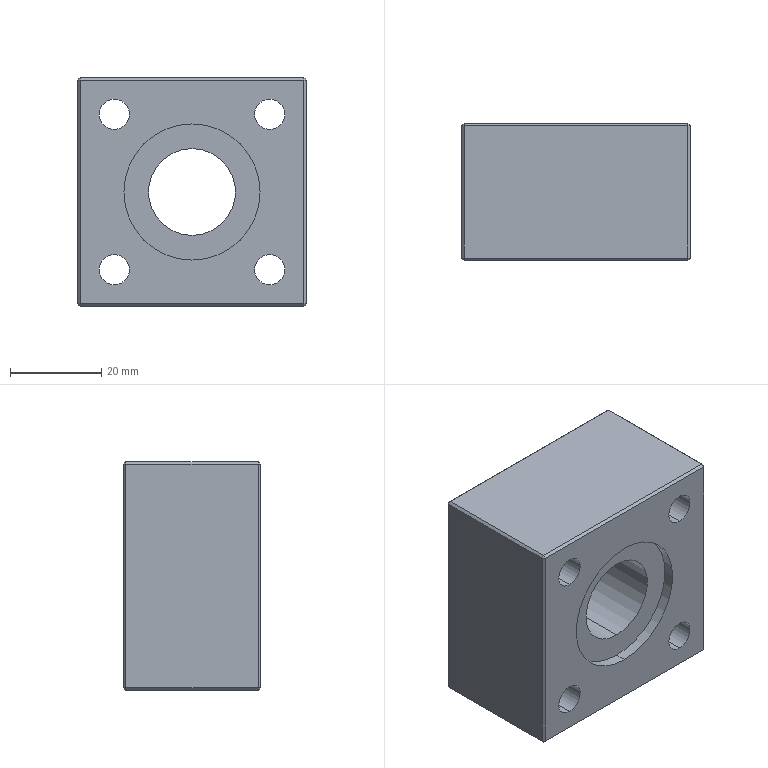Part | SolidWorks | features HoleWzd 2, Chamfer 1, Extrusion 1, ICE 1 | 1 solid | 51 faces | box 50 x 30 x 50 mm | volume 59677 mm3 | plane 31 | cylinder 20 | commonest cylinder face diameters 6.6 x8 11 x8 19 x2 29.8 x2
STEP:
#1=CARTESIAN_POINT('',(0.,2.4,14.9));
#2=VERTEX_POINT('',#1);
#3=CARTESIAN_POINT('',(0.,2.4,-14.9));
#4=VERTEX_POINT('',#3);
#5=CARTESIAN_POINT('',(0.,2.4,0.));
#6=DIRECTION('',(0.,-1.,0.));
#7=DIRECTION('',(0.,0.,-1.));
#8=AXIS2_PLACEMENT_3D('',#5,#6,#7);
#9=CIRCLE('',#8,14.9);
#10=EDGE_CURVE('',#2,#4,#9,.T.);
#11=ORIENTED_EDGE('',*,*,#10,.F.);
#12=CARTESIAN_POINT('',(0.,0.,14.9));
#13=VERTEX_POINT('',#12);
#14=CARTESIAN_POINT('',(0.,2.4,14.9));
#15=DIRECTION('',(0.,-1.,0.));
#16=VECTOR('',#15,1000.);
#17=LINE('',#14,#16);
#18=EDGE_CURVE('',#2,#13,#17,.T.);
#19=ORIENTED_EDGE('',*,*,#18,.T.);
#20=CARTESIAN_POINT('',(0.,0.,-14.9));
#21=VERTEX_POINT('',#20);
#22=CARTESIAN_POINT('',(0.,0.,0.));
#23=DIRECTION('',(0.,-1.,0.));
#24=DIRECTION('',(0.,0.,-1.));
#25=AXIS2_PLACEMENT_3D('',#22,#23,#24);
#26=CIRCLE('',#25,14.9);
#27=EDGE_CURVE('',#13,#21,#26,.T.);
#28=ORIENTED_EDGE('',*,*,#27,.T.);
#29=CARTESIAN_POINT('',(0.,2.4,-14.9));
#30=DIRECTION('',(0.,-1.,0.));
#31=VECTOR('',#30,1000.);
#32=LINE('',#29,#31);
#33=EDGE_CURVE('',#4,#21,#32,.T.);
#34=ORIENTED_EDGE('',*,*,#33,.F.);
#35=EDGE_LOOP('',(#11,#19,#28,#34));
#36=FACE_OUTER_BOUND('',#35,.T.);
#37=CARTESIAN_POINT('',(0.,2.4,0.));
#38=DIRECTION('',(0.,-1.,0.));
#39=DIRECTION('',(0.,0.,-1.));
#40=AXIS2_PLACEMENT_3D('',#37,#38,#39);
#41=CYLINDRICAL_SURFACE('',#40,14.9);
#42=ADVANCED_FACE('',(#36),#41,.F.);
#43=CARTESIAN_POINT('',(17.,23.2,11.5));
#44=VERTEX_POINT('',#43);
#45=CARTESIAN_POINT('',(17.,23.2,22.5));
#46=VERTEX_POINT('',#45);
#47=CARTESIAN_POINT('',(17.,23.2,17.));
#48=DIRECTION('',(0.,1.,0.));
#49=DIRECTION('',(0.,0.,1.));
#50=AXIS2_PLACEMENT_3D('',#47,#48,#49);
#51=CIRCLE('',#50,5.5);
#52=EDGE_CURVE('',#44,#46,#51,.T.);
#53=ORIENTED_EDGE('',*,*,#52,.F.);
#54=CARTESIAN_POINT('',(17.,30.,11.5));
#55=VERTEX_POINT('',#54);
#56=CARTESIAN_POINT('',(17.,30.,11.5));
#57=DIRECTION('',(0.,1.,0.));
#58=VECTOR('',#57,1000.);
#59=LINE('',#56,#58);
#60=EDGE_CURVE('',#44,#55,#59,.T.);
#61=ORIENTED_EDGE('',*,*,#60,.T.);
#62=CARTESIAN_POINT('',(17.,30.,22.5));
#63=VERTEX_POINT('',#62);
#64=CARTESIAN_POINT('',(17.,30.,17.));
#65=DIRECTION('',(0.,1.,0.));
#66=DIRECTION('',(0.,0.,1.));
#67=AXIS2_PLACEMENT_3D('',#64,#65,#66);
#68=CIRCLE('',#67,5.5);
#69=EDGE_CURVE('',#55,#63,#68,.T.);
#70=ORIENTED_EDGE('',*,*,#69,.T.);
#71=CARTESIAN_POINT('',(17.,30.,22.5));
#72=DIRECTION('',(0.,1.,0.));
#73=VECTOR('',#72,1000.);
#74=LINE('',#71,#73);
#75=EDGE_CURVE('',#46,#63,#74,.T.);
#76=ORIENTED_EDGE('',*,*,#75,.F.);
#77=EDGE_LOOP('',(#53,#61,#70,#76));
#78=FACE_OUTER_BOUND('',#77,.T.);
#79=CARTESIAN_POINT('',(17.,30.,17.));
#80=DIRECTION('',(0.,1.,0.));
#81=DIRECTION('',(0.,0.,1.));
#82=AXIS2_PLACEMENT_3D('',#79,#80,#81);
#83=CYLINDRICAL_SURFACE('',#82,5.5);
#84=ADVANCED_FACE('',(#78),#83,.F.);
#85=CARTESIAN_POINT('',(17.,0.,13.7));
#86=VERTEX_POINT('',#85);
#87=CARTESIAN_POINT('',(17.,0.,20.3));
#88=VERTEX_POINT('',#87);
#89=CARTESIAN_POINT('',(17.,0.,17.));
#90=DIRECTION('',(0.,1.,0.));
#91=DIRECTION('',(0.,0.,1.));
#92=AXIS2_PLACEMENT_3D('',#89,#90,#91);
#93=CIRCLE('',#92,3.3);
#94=EDGE_CURVE('',#86,#88,#93,.T.);
#95=ORIENTED_EDGE('',*,*,#94,.F.);
#96=CARTESIAN_POINT('',(17.,23.2,13.7));
#97=VERTEX_POINT('',#96);
#98=CARTESIAN_POINT('',(17.,30.,13.7));
#99=DIRECTION('',(0.,1.,0.));
#100=VECTOR('',#99,1000.);
#101=LINE('',#98,#100);
#102=EDGE_CURVE('',#86,#97,#101,.T.);
#103=ORIENTED_EDGE('',*,*,#102,.T.);
#104=CARTESIAN_POINT('',(17.,23.2,20.3));
#105=VERTEX_POINT('',#104);
#106=CARTESIAN_POINT('',(17.,23.2,17.));
#107=DIRECTION('',(0.,1.,0.));
#108=DIRECTION('',(0.,0.,1.));
#109=AXIS2_PLACEMENT_3D('',#106,#107,#108);
#110=CIRCLE('',#109,3.3);
#111=EDGE_CURVE('',#97,#105,#110,.T.);
#112=ORIENTED_EDGE('',*,*,#111,.T.);
#113=CARTESIAN_POINT('',(17.,30.,20.3));
#114=DIRECTION('',(0.,1.,0.));
#115=VECTOR('',#114,1000.);
#116=LINE('',#113,#115);
#117=EDGE_CURVE('',#88,#105,#116,.T.);
#118=ORIENTED_EDGE('',*,*,#117,.F.);
#119=EDGE_LOOP('',(#95,#103,#112,#118));
#120=FACE_OUTER_BOUND('',#119,.T.);
#121=CARTESIAN_POINT('',(17.,30.,17.));
#122=DIRECTION('',(0.,1.,0.));
#123=DIRECTION('',(0.,0.,1.));
#124=AXIS2_PLACEMENT_3D('',#121,#122,#123);
#125=CYLINDRICAL_SURFACE('',#124,3.3);
#126=ADVANCED_FACE('',(#120),#125,.F.);
#127=CARTESIAN_POINT('',(-17.,23.2,-22.5));
#128=VERTEX_POINT('',#127);
#129=CARTESIAN_POINT('',(-17.,23.2,-11.5));
#130=VERTEX_POINT('',#129);
#131=CARTESIAN_POINT('',(-17.,23.2,-17.));
#132=DIRECTION('',(0.,1.,0.));
#133=DIRECTION('',(0.,0.,1.));
#134=AXIS2_PLACEMENT_3D('',#131,#132,#133);
#135=CIRCLE('',#134,5.5);
#136=EDGE_CURVE('',#128,#130,#135,.T.);
#137=ORIENTED_EDGE('',*,*,#136,.F.);
#138=CARTESIAN_POINT('',(-17.,30.,-22.5));
#139=VERTEX_POINT('',#138);
#140=CARTESIAN_POINT('',(-17.,30.,-22.5));
#141=DIRECTION('',(0.,1.,0.));
#142=VECTOR('',#141,1000.);
#143=LINE('',#140,#142);
#144=EDGE_CURVE('',#128,#139,#143,.T.);
#145=ORIENTED_EDGE('',*,*,#144,.T.);
#146=CARTESIAN_POINT('',(-17.,30.,-11.5));
#147=VERTEX_POINT('',#146);
#148=CARTESIAN_POINT('',(-17.,30.,-17.));
#149=DIRECTION('',(0.,1.,0.));
#150=DIRECTION('',(0.,0.,1.));
#151=AXIS2_PLACEMENT_3D('',#148,#149,#150);
#152=CIRCLE('',#151,5.5);
#153=EDGE_CURVE('',#139,#147,#152,.T.);
#154=ORIENTED_EDGE('',*,*,#153,.T.);
#155=CARTESIAN_POINT('',(-17.,30.,-11.5));
#156=DIRECTION('',(0.,1.,0.));
#157=VECTOR('',#156,1000.);
#158=LINE('',#155,#157);
#159=EDGE_CURVE('',#130,#147,#158,.T.);
#160=ORIENTED_EDGE('',*,*,#159,.F.);
#161=EDGE_LOOP('',(#137,#145,#154,#160));
#162=FACE_OUTER_BOUND('',#161,.T.);
#163=CARTESIAN_POINT('',(-17.,30.,-17.));
#164=DIRECTION('',(0.,1.,0.));
#165=DIRECTION('',(0.,0.,1.));
#166=AXIS2_PLACEMENT_3D('',#163,#164,#165);
#167=CYLINDRICAL_SURFACE('',#166,5.5);
#168=ADVANCED_FACE('',(#162),#167,.F.);
#169=CARTESIAN_POINT('',(-17.,0.,-20.3));
#170=VERTEX_POINT('',#169);
#171=CARTESIAN_POINT('',(-17.,0.,-13.7));
#172=VERTEX_POINT('',#171);
#173=CARTESIAN_POINT('',(-17.,0.,-17.));
#174=DIRECTION('',(0.,1.,0.));
#175=DIRECTION('',(0.,0.,1.));
#176=AXIS2_PLACEMENT_3D('',#173,#174,#175);
#177=CIRCLE('',#176,3.3);
#178=EDGE_CURVE('',#170,#172,#177,.T.);
#179=ORIENTED_EDGE('',*,*,#178,.F.);
#180=CARTESIAN_POINT('',(-17.,23.2,-20.3));
#181=VERTEX_POINT('',#180);
#182=CARTESIAN_POINT('',(-17.,30.,-20.3));
#183=DIRECTION('',(0.,1.,0.));
#184=VECTOR('',#183,1000.);
#185=LINE('',#182,#184);
#186=EDGE_CURVE('',#170,#181,#185,.T.);
#187=ORIENTED_EDGE('',*,*,#186,.T.);
#188=CARTESIAN_POINT('',(-17.,23.2,-13.7));
#189=VERTEX_POINT('',#188);
#190=CARTESIAN_POINT('',(-17.,23.2,-17.));
#191=DIRECTION('',(0.,1.,0.));
#192=DIRECTION('',(0.,0.,1.));
#193=AXIS2_PLACEMENT_3D('',#190,#191,#192);
#194=CIRCLE('',#193,3.3);
#195=EDGE_CURVE('',#181,#189,#194,.T.);
#196=ORIENTED_EDGE('',*,*,#195,.T.);
#197=CARTESIAN_POINT('',(-17.,30.,-13.7));
#198=DIRECTION('',(0.,1.,0.));
#199=VECTOR('',#198,1000.);
#200=LINE('',#197,#199);
#201=EDGE_CURVE('',#172,#189,#200,.T.);
#202=ORIENTED_EDGE('',*,*,#201,.F.);
#203=EDGE_LOOP('',(#179,#187,#196,#202));
#204=FACE_OUTER_BOUND('',#203,.T.);
#205=CARTESIAN_POINT('',(-17.,30.,-17.));
#206=DIRECTION('',(0.,1.,0.));
#207=DIRECTION('',(0.,0.,1.));
#208=AXIS2_PLACEMENT_3D('',#205,#206,#207);
#209=CYLINDRICAL_SURFACE('',#208,3.3);
#210=ADVANCED_FACE('',(#204),#209,.F.);
#211=CARTESIAN_POINT('',(-17.,23.2,11.5));
#212=VERTEX_POINT('',#211);
#213=CARTESIAN_POINT('',(-17.,23.2,22.5));
#214=VERTEX_POINT('',#213);
#215=CARTESIAN_POINT('',(-17.,23.2,17.));
#216=DIRECTION('',(0.,1.,0.));
#217=DIRECTION('',(0.,0.,1.));
#218=AXIS2_PLACEMENT_3D('',#215,#216,#217);
#219=CIRCLE('',#218,5.5);
#220=EDGE_CURVE('',#212,#214,#219,.T.);
#221=ORIENTED_EDGE('',*,*,#220,.F.);
#222=CARTESIAN_POINT('',(-17.,30.,11.5));
#223=VERTEX_POINT('',#222);
#224=CARTESIAN_POINT('',(-17.,30.,11.5));
#225=DIRECTION('',(0.,1.,0.));
#226=VECTOR('',#225,1000.);
#227=LINE('',#224,#226);
#228=EDGE_CURVE('',#212,#223,#227,.T.);
#229=ORIENTED_EDGE('',*,*,#228,.T.);
#230=CARTESIAN_POINT('',(-17.,30.,22.5));
#231=VERTEX_POINT('',#230);
#232=CARTESIAN_POINT('',(-17.,30.,17.));
#233=DIRECTION('',(0.,1.,0.));
#234=DIRECTION('',(0.,0.,1.));
#235=AXIS2_PLACEMENT_3D('',#232,#233,#234);
#236=CIRCLE('',#235,5.5);
#237=EDGE_CURVE('',#223,#231,#236,.T.);
#238=ORIENTED_EDGE('',*,*,#237,.T.);
#239=CARTESIAN_POINT('',(-17.,30.,22.5));
#240=DIRECTION('',(0.,1.,0.));
#241=VECTOR('',#240,1000.);
#242=LINE('',#239,#241);
#243=EDGE_CURVE('',#214,#231,#242,.T.);
#244=ORIENTED_EDGE('',*,*,#243,.F.);
#245=EDGE_LOOP('',(#221,#229,#238,#244));
#246=FACE_OUTER_BOUND('',#245,.T.);
#247=CARTESIAN_POINT('',(-17.,30.,17.));
#248=DIRECTION('',(0.,1.,0.));
#249=DIRECTION('',(0.,0.,1.));
#250=AXIS2_PLACEMENT_3D('',#247,#248,#249);
#251=CYLINDRICAL_SURFACE('',#250,5.5);
#252=ADVANCED_FACE('',(#246),#251,.F.);
#253=CARTESIAN_POINT('',(-17.,0.,13.7));
#254=VERTEX_POINT('',#253);
#255=CARTESIAN_POINT('',(-17.,0.,20.3));
#256=VERTEX_POINT('',#255);
#257=CARTESIAN_POINT('',(-17.,0.,17.));
#258=DIRECTION('',(0.,1.,0.));
#259=DIRECTION('',(0.,0.,1.));
#260=AXIS2_PLACEMENT_3D('',#257,#258,#259);
#261=CIRCLE('',#260,3.3);
#262=EDGE_CURVE('',#254,#256,#261,.T.);
#263=ORIENTED_EDGE('',*,*,#262,.F.);
#264=CARTESIAN_POINT('',(-17.,23.2,13.7));
#265=VERTEX_POINT('',#264);
#266=CARTESIAN_POINT('',(-17.,30.,13.7));
#267=DIRECTION('',(0.,1.,0.));
#268=VECTOR('',#267,1000.);
#269=LINE('',#266,#268);
#270=EDGE_CURVE('',#254,#265,#269,.T.);
#271=ORIENTED_EDGE('',*,*,#270,.T.);
#272=CARTESIAN_POINT('',(-17.,23.2,20.3));
#273=VERTEX_POINT('',#272);
#274=CARTESIAN_POINT('',(-17.,23.2,17.));
#275=DIRECTION('',(0.,1.,0.));
#276=DIRECTION('',(0.,0.,1.));
#277=AXIS2_PLACEMENT_3D('',#274,#275,#276);
#278=CIRCLE('',#277,3.3);
#279=EDGE_CURVE('',#265,#273,#278,.T.);
#280=ORIENTED_EDGE('',*,*,#279,.T.);
#281=CARTESIAN_POINT('',(-17.,30.,20.3));
#282=DIRECTION('',(0.,1.,0.));
#283=VECTOR('',#282,1000.);
#284=LINE('',#281,#283);
#285=EDGE_CURVE('',#256,#273,#284,.T.);
#286=ORIENTED_EDGE('',*,*,#285,.F.);
#287=EDGE_LOOP('',(#263,#271,#280,#286));
#288=FACE_OUTER_BOUND('',#287,.T.);
#289=CARTESIAN_POINT('',(-17.,30.,17.));
#290=DIRECTION('',(0.,1.,0.));
#291=DIRECTION('',(0.,0.,1.));
#292=AXIS2_PLACEMENT_3D('',#289,#290,#291);
#293=CYLINDRICAL_SURFACE('',#292,3.3);
#294=ADVANCED_FACE('',(#288),#293,.F.);
#295=CARTESIAN_POINT('',(17.,23.2,-22.5));
#296=VERTEX_POINT('',#295);
#297=CARTESIAN_POINT('',(17.,23.2,-11.5));
#298=VERTEX_POINT('',#297);
#299=CARTESIAN_POINT('',(17.,23.2,-17.));
#300=DIRECTION('',(0.,1.,0.));
#301=DIRECTION('',(0.,0.,1.));
#302=AXIS2_PLACEMENT_3D('',#299,#300,#301);
#303=CIRCLE('',#302,5.5);
#304=EDGE_CURVE('',#296,#298,#303,.T.);
#305=ORIENTED_EDGE('',*,*,#304,.F.);
#306=CARTESIAN_POINT('',(17.,30.,-22.5));
#307=VERTEX_POINT('',#306);
#308=CARTESIAN_POINT('',(17.,30.,-22.5));
#309=DIRECTION('',(0.,1.,0.));
#310=VECTOR('',#309,1000.);
#311=LINE('',#308,#310);
#312=EDGE_CURVE('',#296,#307,#311,.T.);
#313=ORIENTED_EDGE('',*,*,#312,.T.);
#314=CARTESIAN_POINT('',(17.,30.,-11.5));
#315=VERTEX_POINT('',#314);
#316=CARTESIAN_POINT('',(17.,30.,-17.));
#317=DIRECTION('',(0.,1.,0.));
#318=DIRECTION('',(0.,0.,1.));
#319=AXIS2_PLACEMENT_3D('',#316,#317,#318);
#320=CIRCLE('',#319,5.5);
#321=EDGE_CURVE('',#307,#315,#320,.T.);
#322=ORIENTED_EDGE('',*,*,#321,.T.);
#323=CARTESIAN_POINT('',(17.,30.,-11.5));
#324=DIRECTION('',(0.,1.,0.));
#325=VECTOR('',#324,1000.);
#326=LINE('',#323,#325);
#327=EDGE_CURVE('',#298,#315,#326,.T.);
#328=ORIENTED_EDGE('',*,*,#327,.F.);
#329=EDGE_LOOP('',(#305,#313,#322,#328));
#330=FACE_OUTER_BOUND('',#329,.T.);
#331=CARTESIAN_POINT('',(17.,30.,-17.));
#332=DIRECTION('',(0.,1.,0.));
#333=DIRECTION('',(0.,0.,1.));
#334=AXIS2_PLACEMENT_3D('',#331,#332,#333);
#335=CYLINDRICAL_SURFACE('',#334,5.5);
#336=ADVANCED_FACE('',(#330),#335,.F.);
#337=CARTESIAN_POINT('',(17.,0.,-20.3));
#338=VERTEX_POINT('',#337);
#339=CARTESIAN_POINT('',(17.,0.,-13.7));
#340=VERTEX_POINT('',#339);
#341=CARTESIAN_POINT('',(17.,0.,-17.));
#342=DIRECTION('',(0.,1.,0.));
#343=DIRECTION('',(0.,0.,1.));
#344=AXIS2_PLACEMENT_3D('',#341,#342,#343);
#345=CIRCLE('',#344,3.3);
#346=EDGE_CURVE('',#338,#340,#345,.T.);
#347=ORIENTED_EDGE('',*,*,#346,.F.);
#348=CARTESIAN_POINT('',(17.,23.2,-20.3));
#349=VERTEX_POINT('',#348);
#350=CARTESIAN_POINT('',(17.,30.,-20.3));
#351=DIRECTION('',(0.,1.,0.));
#352=VECTOR('',#351,1000.);
#353=LINE('',#350,#352);
#354=EDGE_CURVE('',#338,#349,#353,.T.);
#355=ORIENTED_EDGE('',*,*,#354,.T.);
#356=CARTESIAN_POINT('',(17.,23.2,-13.7));
#357=VERTEX_POINT('',#356);
#358=CARTESIAN_POINT('',(17.,23.2,-17.));
#359=DIRECTION('',(0.,1.,0.));
#360=DIRECTION('',(0.,0.,1.));
#361=AXIS2_PLACEMENT_3D('',#358,#359,#360);
#362=CIRCLE('',#361,3.3);
#363=EDGE_CURVE('',#349,#357,#362,.T.);
#364=ORIENTED_EDGE('',*,*,#363,.T.);
#365=CARTESIAN_POINT('',(17.,30.,-13.7));
#366=DIRECTION('',(0.,1.,0.));
#367=VECTOR('',#366,1000.);
#368=LINE('',#365,#367);
#369=EDGE_CURVE('',#340,#357,#368,.T.);
#370=ORIENTED_EDGE('',*,*,#369,.F.);
#371=EDGE_LOOP('',(#347,#355,#364,#370));
#372=FACE_OUTER_BOUND('',#371,.T.);
#373=CARTESIAN_POINT('',(17.,30.,-17.));
#374=DIRECTION('',(0.,1.,0.));
#375=DIRECTION('',(0.,0.,1.));
#376=AXIS2_PLACEMENT_3D('',#373,#374,#375);
#377=CYLINDRICAL_SURFACE('',#376,3.3);
#378=ADVANCED_FACE('',(#372),#377,.F.);
#379=CARTESIAN_POINT('',(0.,2.4,-9.5));
#380=VERTEX_POINT('',#379);
#381=CARTESIAN_POINT('',(0.,2.4,9.5));
#382=VERTEX_POINT('',#381);
#383=CARTESIAN_POINT('',(0.,2.4,0.));
#384=DIRECTION('',(0.,1.,0.));
#385=DIRECTION('',(0.,0.,-1.));
#386=AXIS2_PLACEMENT_3D('',#383,#384,#385);
#387=CIRCLE('',#386,9.5);
#388=EDGE_CURVE('',#380,#382,#387,.T.);
#389=ORIENTED_EDGE('',*,*,#388,.F.);
#390=CARTESIAN_POINT('',(0.,30.,-9.5));
#391=VERTEX_POINT('',#390);
#392=CARTESIAN_POINT('',(0.,30.,-9.5));
#393=DIRECTION('',(0.,1.,0.));
#394=VECTOR('',#393,1000.);
#395=LINE('',#392,#394);
#396=EDGE_CURVE('',#380,#391,#395,.T.);
#397=ORIENTED_EDGE('',*,*,#396,.T.);
#398=CARTESIAN_POINT('',(0.,30.,9.5));
#399=VERTEX_POINT('',#398);
#400=CARTESIAN_POINT('',(0.,30.,0.));
#401=DIRECTION('',(0.,1.,0.));
#402=DIRECTION('',(0.,0.,1.));
#403=AXIS2_PLACEMENT_3D('',#400,#401,#402);
#404=CIRCLE('',#403,9.5);
#405=EDGE_CURVE('',#391,#399,#404,.T.);
#406=ORIENTED_EDGE('',*,*,#405,.T.);
#407=CARTESIAN_POINT('',(0.,30.,9.5));
#408=DIRECTION('',(0.,1.,0.));
#409=VECTOR('',#408,1000.);
#410=LINE('',#407,#409);
#411=EDGE_CURVE('',#382,#399,#410,.T.);
#412=ORIENTED_EDGE('',*,*,#411,.F.);
#413=EDGE_LOOP('',(#389,#397,#406,#412));
#414=FACE_OUTER_BOUND('',#413,.T.);
#415=CARTESIAN_POINT('',(0.,30.,0.));
#416=DIRECTION('',(0.,1.,0.));
#417=DIRECTION('',(0.,0.,1.));
#418=AXIS2_PLACEMENT_3D('',#415,#416,#417);
#419=CYLINDRICAL_SURFACE('',#418,9.5);
#420=ADVANCED_FACE('',(#414),#419,.F.);
#421=ORIENTED_EDGE('',*,*,#396,.F.);
#422=CARTESIAN_POINT('',(0.,2.4,0.));
#423=DIRECTION('',(0.,1.,0.));
#424=DIRECTION('',(0.,0.,-1.));
#425=AXIS2_PLACEMENT_3D('',#422,#423,#424);
#426=CIRCLE('',#425,9.5);
#427=EDGE_CURVE('',#382,#380,#426,.T.);
#428=ORIENTED_EDGE('',*,*,#427,.F.);
#429=ORIENTED_EDGE('',*,*,#411,.T.);
#430=CARTESIAN_POINT('',(0.,30.,0.));
#431=DIRECTION('',(0.,1.,0.));
#432=DIRECTION('',(0.,0.,1.));
#433=AXIS2_PLACEMENT_3D('',#430,#431,#432);
#434=CIRCLE('',#433,9.5);
#435=EDGE_CURVE('',#399,#391,#434,.T.);
#436=ORIENTED_EDGE('',*,*,#435,.T.);
#437=EDGE_LOOP('',(#421,#428,#429,#436));
#438=FACE_OUTER_BOUND('',#437,.T.);
#439=CARTESIAN_POINT('',(0.,30.,0.));
#440=DIRECTION('',(0.,1.,0.));
#441=DIRECTION('',(0.,0.,1.));
#442=AXIS2_PLACEMENT_3D('',#439,#440,#441);
#443=CYLINDRICAL_SURFACE('',#442,9.5);
#444=ADVANCED_FACE('',(#438),#443,.F.);
#445=CARTESIAN_POINT('',(25.,0.5,-24.5));
#446=VERTEX_POINT('',#445);
#447=CARTESIAN_POINT('',(25.,29.5,-24.5));
#448=VERTEX_POINT('',#447);
#449=CARTESIAN_POINT('',(25.,30.,-24.5));
#450=DIRECTION('',(0.,1.,0.));
#451=VECTOR('',#450,1000.);
#452=LINE('',#449,#451);
#453=EDGE_CURVE('',#446,#448,#452,.T.);
#454=ORIENTED_EDGE('',*,*,#453,.T.);
#455=CARTESIAN_POINT('',(25.,29.5,24.5));
#456=VERTEX_POINT('',#455);
#457=CARTESIAN_POINT('',(25.,29.5,25.));
#458=DIRECTION('',(0.,0.,1.));
#459=VECTOR('',#458,1000.);
#460=LINE('',#457,#459);
#461=EDGE_CURVE('',#448,#456,#460,.T.);
#462=ORIENTED_EDGE('',*,*,#461,.T.);
#463=CARTESIAN_POINT('',(25.,0.5,24.5));
#464=VERTEX_POINT('',#463);
#465=CARTESIAN_POINT('',(25.,30.,24.5));
#466=DIRECTION('',(0.,-1.,0.));
#467=VECTOR('',#466,1000.);
#468=LINE('',#465,#467);
#469=EDGE_CURVE('',#456,#464,#468,.T.);
#470=ORIENTED_EDGE('',*,*,#469,.T.);
#471=CARTESIAN_POINT('',(25.,0.5,-25.));
#472=DIRECTION('',(0.,0.,-1.));
#473=VECTOR('',#472,1000.);
#474=LINE('',#471,#473);
#475=EDGE_CURVE('',#464,#446,#474,.T.);
#476=ORIENTED_EDGE('',*,*,#475,.T.);
#477=EDGE_LOOP('',(#454,#462,#470,#476));
#478=FACE_OUTER_BOUND('',#477,.T.);
#479=CARTESIAN_POINT('',(25.,30.,-25.));
#480=DIRECTION('',(-1.,0.,0.));
#481=DIRECTION('',(0.,0.,1.));
#482=AXIS2_PLACEMENT_3D('',#479,#480,#481);
#483=PLANE('',#482);
#484=ADVANCED_FACE('',(#478),#483,.F.);
#485=CARTESIAN_POINT('',(-24.5,0.5,-25.));
#486=VERTEX_POINT('',#485);
#487=CARTESIAN_POINT('',(-24.5,29.5,-25.));
#488=VERTEX_POINT('',#487);
#489=CARTESIAN_POINT('',(-24.5,30.,-25.));
#490=DIRECTION('',(0.,1.,0.));
#491=VECTOR('',#490,1000.);
#492=LINE('',#489,#491);
#493=EDGE_CURVE('',#486,#488,#492,.T.);
#494=ORIENTED_EDGE('',*,*,#493,.T.);
#495=CARTESIAN_POINT('',(24.5,29.5,-25.));
#496=VERTEX_POINT('',#495);
#497=CARTESIAN_POINT('',(25.,29.5,-25.));
#498=DIRECTION('',(1.,0.,0.));
#499=VECTOR('',#498,1000.);
#500=LINE('',#497,#499);
#501=EDGE_CURVE('',#488,#496,#500,.T.);
#502=ORIENTED_EDGE('',*,*,#501,.T.);
#503=CARTESIAN_POINT('',(24.5,0.5,-25.));
#504=VERTEX_POINT('',#503);
#505=CARTESIAN_POINT('',(24.5,30.,-25.));
#506=DIRECTION('',(0.,-1.,0.));
#507=VECTOR('',#506,1000.);
#508=LINE('',#505,#507);
#509=EDGE_CURVE('',#496,#504,#508,.T.);
#510=ORIENTED_EDGE('',*,*,#509,.T.);
#511=CARTESIAN_POINT('',(-25.,0.5,-25.));
#512=DIRECTION('',(-1.,0.,0.));
#513=VECTOR('',#512,1000.);
#514=LINE('',#511,#513);
#515=EDGE_CURVE('',#504,#486,#514,.T.);
#516=ORIENTED_EDGE('',*,*,#515,.T.);
#517=EDGE_LOOP('',(#494,#502,#510,#516));
#518=FACE_OUTER_BOUND('',#517,.T.);
#519=CARTESIAN_POINT('',(-25.,30.,-25.));
#520=DIRECTION('',(0.,0.,1.));
#521=DIRECTION('',(1.,0.,0.));
#522=AXIS2_PLACEMENT_3D('',#519,#520,#521);
#523=PLANE('',#522);
#524=ADVANCED_FACE('',(#518),#523,.F.);
#525=CARTESIAN_POINT('',(-25.,29.5,24.5));
#526=VERTEX_POINT('',#525);
#527=CARTESIAN_POINT('',(-25.,29.5,-24.5));
#528=VERTEX_POINT('',#527);
#529=CARTESIAN_POINT('',(-25.,29.5,-25.));
#530=DIRECTION('',(0.,0.,-1.));
#531=VECTOR('',#530,1000.);
#532=LINE('',#529,#531);
#533=EDGE_CURVE('',#526,#528,#532,.T.);
#534=ORIENTED_EDGE('',*,*,#533,.T.);
#535=CARTESIAN_POINT('',(-25.,0.5,-24.5));
#536=VERTEX_POINT('',#535);
#537=CARTESIAN_POINT('',(-25.,30.,-24.5));
#538=DIRECTION('',(0.,-1.,0.));
#539=VECTOR('',#538,1000.);
#540=LINE('',#537,#539);
#541=EDGE_CURVE('',#528,#536,#540,.T.);
#542=ORIENTED_EDGE('',*,*,#541,.T.);
#543=CARTESIAN_POINT('',(-25.,0.5,24.5));
#544=VERTEX_POINT('',#543);
#545=CARTESIAN_POINT('',(-25.,0.5,-25.));
#546=DIRECTION('',(0.,0.,1.));
#547=VECTOR('',#546,1000.);
#548=LINE('',#545,#547);
#549=EDGE_CURVE('',#536,#544,#548,.T.);
#550=ORIENTED_EDGE('',*,*,#549,.T.);
#551=CARTESIAN_POINT('',(-25.,30.,24.5));
#552=DIRECTION('',(0.,1.,0.));
#553=VECTOR('',#552,1000.);
#554=LINE('',#551,#553);
#555=EDGE_CURVE('',#544,#526,#554,.T.);
#556=ORIENTED_EDGE('',*,*,#555,.T.);
#557=EDGE_LOOP('',(#534,#542,#550,#556));
#558=FACE_OUTER_BOUND('',#557,.T.);
#559=CARTESIAN_POINT('',(-25.,30.,-25.));
#560=DIRECTION('',(1.,0.,0.));
#561=DIRECTION('',(0.,0.,-1.));
#562=AXIS2_PLACEMENT_3D('',#559,#560,#561);
#563=PLANE('',#562);
#564=ADVANCED_FACE('',(#558),#563,.F.);
#565=CARTESIAN_POINT('',(24.5,29.5,25.));
#566=VERTEX_POINT('',#565);
#567=CARTESIAN_POINT('',(-24.5,29.5,25.));
#568=VERTEX_POINT('',#567);
#569=CARTESIAN_POINT('',(-25.,29.5,25.));
#570=DIRECTION('',(-1.,0.,0.));
#571=VECTOR('',#570,1000.);
#572=LINE('',#569,#571);
#573=EDGE_CURVE('',#566,#568,#572,.T.);
#574=ORIENTED_EDGE('',*,*,#573,.T.);
#575=CARTESIAN_POINT('',(-24.5,0.5,25.));
#576=VERTEX_POINT('',#575);
#577=CARTESIAN_POINT('',(-24.5,30.,25.));
#578=DIRECTION('',(0.,-1.,0.));
#579=VECTOR('',#578,1000.);
#580=LINE('',#577,#579);
#581=EDGE_CURVE('',#568,#576,#580,.T.);
#582=ORIENTED_EDGE('',*,*,#581,.T.);
#583=CARTESIAN_POINT('',(24.5,0.5,25.));
#584=VERTEX_POINT('',#583);
#585=CARTESIAN_POINT('',(-25.,0.5,25.));
#586=DIRECTION('',(1.,0.,0.));
#587=VECTOR('',#586,1000.);
#588=LINE('',#585,#587);
#589=EDGE_CURVE('',#576,#584,#588,.T.);
#590=ORIENTED_EDGE('',*,*,#589,.T.);
#591=CARTESIAN_POINT('',(24.5,30.,25.));
#592=DIRECTION('',(0.,1.,0.));
#593=VECTOR('',#592,1000.);
#594=LINE('',#591,#593);
#595=EDGE_CURVE('',#584,#566,#594,.T.);
#596=ORIENTED_EDGE('',*,*,#595,.T.);
#597=EDGE_LOOP('',(#574,#582,#590,#596));
#598=FACE_OUTER_BOUND('',#597,.T.);
#599=CARTESIAN_POINT('',(-25.,30.,25.));
#600=DIRECTION('',(0.,0.,-1.));
#601=DIRECTION('',(-1.,0.,0.));
#602=AXIS2_PLACEMENT_3D('',#599,#600,#601);
#603=PLANE('',#602);
#604=ADVANCED_FACE('',(#598),#603,.F.);
#605=CARTESIAN_POINT('',(24.5,30.,-24.5));
#606=VERTEX_POINT('',#605);
#607=CARTESIAN_POINT('',(-24.5,30.,-24.5));
#608=VERTEX_POINT('',#607);
#609=CARTESIAN_POINT('',(-25.,30.,-24.5));
#610=DIRECTION('',(-1.,0.,0.));
#611=VECTOR('',#610,1000.);
#612=LINE('',#609,#611);
#613=EDGE_CURVE('',#606,#608,#612,.T.);
#614=ORIENTED_EDGE('',*,*,#613,.T.);
#615=CARTESIAN_POINT('',(-24.5,30.,24.5));
#616=VERTEX_POINT('',#615);
#617=CARTESIAN_POINT('',(-24.5,30.,25.));
#618=DIRECTION('',(0.,0.,1.));
#619=VECTOR('',#618,1000.);
#620=LINE('',#617,#619);
#621=EDGE_CURVE('',#608,#616,#620,.T.);
#622=ORIENTED_EDGE('',*,*,#621,.T.);
#623=CARTESIAN_POINT('',(24.5,30.,24.5));
#624=VERTEX_POINT('',#623);
#625=CARTESIAN_POINT('',(25.,30.,24.5));
#626=DIRECTION('',(1.,0.,0.));
#627=VECTOR('',#626,1000.);
#628=LINE('',#625,#627);
#629=EDGE_CURVE('',#616,#624,#628,.T.);
#630=ORIENTED_EDGE('',*,*,#629,.T.);
#631=CARTESIAN_POINT('',(24.5,30.,-25.));
#632=DIRECTION('',(0.,0.,-1.));
#633=VECTOR('',#632,1000.);
#634=LINE('',#631,#633);
#635=EDGE_CURVE('',#624,#606,#634,.T.);
#636=ORIENTED_EDGE('',*,*,#635,.T.);
#637=EDGE_LOOP('',(#614,#622,#630,#636));
#638=FACE_OUTER_BOUND('',#637,.T.);
#639=ORIENTED_EDGE('',*,*,#435,.F.);
#640=ORIENTED_EDGE('',*,*,#405,.F.);
#641=EDGE_LOOP('',(#639,#640));
#642=FACE_BOUND('',#641,.T.);
#643=CARTESIAN_POINT('',(17.,30.,17.));
#644=DIRECTION('',(0.,1.,0.));
#645=DIRECTION('',(0.,0.,1.));
#646=AXIS2_PLACEMENT_3D('',#643,#644,#645);
#647=CIRCLE('',#646,5.5);
#648=EDGE_CURVE('',#63,#55,#647,.T.);
#649=ORIENTED_EDGE('',*,*,#648,.F.);
#650=ORIENTED_EDGE('',*,*,#69,.F.);
#651=EDGE_LOOP('',(#649,#650));
#652=FACE_BOUND('',#651,.T.);
#653=CARTESIAN_POINT('',(-17.,30.,-17.));
#654=DIRECTION('',(0.,1.,0.));
#655=DIRECTION('',(0.,0.,1.));
#656=AXIS2_PLACEMENT_3D('',#653,#654,#655);
#657=CIRCLE('',#656,5.5);
#658=EDGE_CURVE('',#147,#139,#657,.T.);
#659=ORIENTED_EDGE('',*,*,#658,.F.);
#660=ORIENTED_EDGE('',*,*,#153,.F.);
#661=EDGE_LOOP('',(#659,#660));
#662=FACE_BOUND('',#661,.T.);
#663=CARTESIAN_POINT('',(-17.,30.,17.));
#664=DIRECTION('',(0.,1.,0.));
#665=DIRECTION('',(0.,0.,1.));
#666=AXIS2_PLACEMENT_3D('',#663,#664,#665);
#667=CIRCLE('',#666,5.5);
#668=EDGE_CURVE('',#231,#223,#667,.T.);
#669=ORIENTED_EDGE('',*,*,#668,.F.);
#670=ORIENTED_EDGE('',*,*,#237,.F.);
#671=EDGE_LOOP('',(#669,#670));
#672=FACE_BOUND('',#671,.T.);
#673=CARTESIAN_POINT('',(17.,30.,-17.));
#674=DIRECTION('',(0.,1.,0.));
#675=DIRECTION('',(0.,0.,1.));
#676=AXIS2_PLACEMENT_3D('',#673,#674,#675);
#677=CIRCLE('',#676,5.5);
#678=EDGE_CURVE('',#315,#307,#677,.T.);
#679=ORIENTED_EDGE('',*,*,#678,.F.);
#680=ORIENTED_EDGE('',*,*,#321,.F.);
#681=EDGE_LOOP('',(#679,#680));
#682=FACE_BOUND('',#681,.T.);
#683=CARTESIAN_POINT('',(0.,30.,0.));
#684=DIRECTION('',(0.,1.,0.));
#685=DIRECTION('',(0.,0.,1.));
#686=AXIS2_PLACEMENT_3D('',#683,#684,#685);
#687=PLANE('',#686);
#688=ADVANCED_FACE('',(#638,#642,#652,#662,#672,#682),#687,.T.);
#689=CARTESIAN_POINT('',(24.5,0.,24.5));
#690=VERTEX_POINT('',#689);
#691=CARTESIAN_POINT('',(-24.5,0.,24.5));
#692=VERTEX_POINT('',#691);
#693=CARTESIAN_POINT('',(0.,0.,24.5));
#694=DIRECTION('',(-1.,0.,0.));
#695=VECTOR('',#694,1000.);
#696=LINE('',#693,#695);
#697=EDGE_CURVE('',#690,#692,#696,.T.);
#698=ORIENTED_EDGE('',*,*,#697,.T.);
#699=CARTESIAN_POINT('',(-24.5,0.,-24.5));
#700=VERTEX_POINT('',#699);
#701=CARTESIAN_POINT('',(-24.5,0.,0.));
#702=DIRECTION('',(0.,0.,-1.));
#703=VECTOR('',#702,1000.);
#704=LINE('',#701,#703);
#705=EDGE_CURVE('',#692,#700,#704,.T.);
#706=ORIENTED_EDGE('',*,*,#705,.T.);
#707=CARTESIAN_POINT('',(24.5,0.,-24.5));
#708=VERTEX_POINT('',#707);
#709=CARTESIAN_POINT('',(0.,0.,-24.5));
#710=DIRECTION('',(1.,0.,0.));
#711=VECTOR('',#710,1000.);
#712=LINE('',#709,#711);
#713=EDGE_CURVE('',#700,#708,#712,.T.);
#714=ORIENTED_EDGE('',*,*,#713,.T.);
#715=CARTESIAN_POINT('',(24.5,0.,0.));
#716=DIRECTION('',(0.,0.,1.));
#717=VECTOR('',#716,1000.);
#718=LINE('',#715,#717);
#719=EDGE_CURVE('',#708,#690,#718,.T.);
#720=ORIENTED_EDGE('',*,*,#719,.T.);
#721=EDGE_LOOP('',(#698,#706,#714,#720));
#722=FACE_OUTER_BOUND('',#721,.T.);
#723=CARTESIAN_POINT('',(0.,0.,0.));
#724=DIRECTION('',(0.,-1.,0.));
#725=DIRECTION('',(0.,0.,-1.));
#726=AXIS2_PLACEMENT_3D('',#723,#724,#725);
#727=CIRCLE('',#726,14.9);
#728=EDGE_CURVE('',#21,#13,#727,.T.);
#729=ORIENTED_EDGE('',*,*,#728,.F.);
#730=ORIENTED_EDGE('',*,*,#27,.F.);
#731=EDGE_LOOP('',(#729,#730));
#732=FACE_BOUND('',#731,.T.);
#733=CARTESIAN_POINT('',(17.,0.,17.));
#734=DIRECTION('',(0.,1.,0.));
#735=DIRECTION('',(0.,0.,1.));
#736=AXIS2_PLACEMENT_3D('',#733,#734,#735);
#737=CIRCLE('',#736,3.3);
#738=EDGE_CURVE('',#88,#86,#737,.T.);
#739=ORIENTED_EDGE('',*,*,#738,.T.);
#740=ORIENTED_EDGE('',*,*,#94,.T.);
#741=EDGE_LOOP('',(#739,#740));
#742=FACE_BOUND('',#741,.T.);
#743=CARTESIAN_POINT('',(-17.,0.,-17.));
#744=DIRECTION('',(0.,1.,0.));
#745=DIRECTION('',(0.,0.,1.));
#746=AXIS2_PLACEMENT_3D('',#743,#744,#745);
#747=CIRCLE('',#746,3.3);
#748=EDGE_CURVE('',#172,#170,#747,.T.);
#749=ORIENTED_EDGE('',*,*,#748,.T.);
#750=ORIENTED_EDGE('',*,*,#178,.T.);
#751=EDGE_LOOP('',(#749,#750));
#752=FACE_BOUND('',#751,.T.);
#753=CARTESIAN_POINT('',(-17.,0.,17.));
#754=DIRECTION('',(0.,1.,0.));
#755=DIRECTION('',(0.,0.,1.));
#756=AXIS2_PLACEMENT_3D('',#753,#754,#755);
#757=CIRCLE('',#756,3.3);
#758=EDGE_CURVE('',#256,#254,#757,.T.);
#759=ORIENTED_EDGE('',*,*,#758,.T.);
#760=ORIENTED_EDGE('',*,*,#262,.T.);
#761=EDGE_LOOP('',(#759,#760));
#762=FACE_BOUND('',#761,.T.);
#763=CARTESIAN_POINT('',(17.,0.,-17.));
#764=DIRECTION('',(0.,1.,0.));
#765=DIRECTION('',(0.,0.,1.));
#766=AXIS2_PLACEMENT_3D('',#763,#764,#765);
#767=CIRCLE('',#766,3.3);
#768=EDGE_CURVE('',#340,#338,#767,.T.);
#769=ORIENTED_EDGE('',*,*,#768,.T.);
#770=ORIENTED_EDGE('',*,*,#346,.T.);
#771=EDGE_LOOP('',(#769,#770));
#772=FACE_BOUND('',#771,.T.);
#773=CARTESIAN_POINT('',(0.,0.,0.));
#774=DIRECTION('',(0.,1.,0.));
#775=DIRECTION('',(0.,0.,1.));
#776=AXIS2_PLACEMENT_3D('',#773,#774,#775);
#777=PLANE('',#776);
#778=ADVANCED_FACE('',(#722,#732,#742,#752,#762,#772),#777,.F.);
#779=ORIENTED_EDGE('',*,*,#354,.F.);
#780=ORIENTED_EDGE('',*,*,#768,.F.);
#781=ORIENTED_EDGE('',*,*,#369,.T.);
#782=CARTESIAN_POINT('',(17.,23.2,-17.));
#783=DIRECTION('',(0.,1.,0.));
#784=DIRECTION('',(0.,0.,1.));
#785=AXIS2_PLACEMENT_3D('',#782,#783,#784);
#786=CIRCLE('',#785,3.3);
#787=EDGE_CURVE('',#357,#349,#786,.T.);
#788=ORIENTED_EDGE('',*,*,#787,.T.);
#789=EDGE_LOOP('',(#779,#780,#781,#788));
#790=FACE_OUTER_BOUND('',#789,.T.);
#791=CARTESIAN_POINT('',(17.,30.,-17.));
#792=DIRECTION('',(0.,1.,0.));
#793=DIRECTION('',(0.,0.,1.));
#794=AXIS2_PLACEMENT_3D('',#791,#792,#793);
#795=CYLINDRICAL_SURFACE('',#794,3.3);
#796=ADVANCED_FACE('',(#790),#795,.F.);
#797=ORIENTED_EDGE('',*,*,#787,.F.);
#798=ORIENTED_EDGE('',*,*,#363,.F.);
#799=EDGE_LOOP('',(#797,#798));
#800=FACE_BOUND('',#799,.T.);
#801=CARTESIAN_POINT('',(17.,23.2,-17.));
#802=DIRECTION('',(0.,1.,0.));
#803=DIRECTION('',(0.,0.,1.));
#804=AXIS2_PLACEMENT_3D('',#801,#802,#803);
#805=CIRCLE('',#804,5.5);
#806=EDGE_CURVE('',#298,#296,#805,.T.);
#807=ORIENTED_EDGE('',*,*,#806,.T.);
#808=ORIENTED_EDGE('',*,*,#304,.T.);
#809=EDGE_LOOP('',(#807,#808));
#810=FACE_OUTER_BOUND('',#809,.T.);
#811=CARTESIAN_POINT('',(20.3,23.2,-17.));
#812=DIRECTION('',(0.,-1.,0.));
#813=DIRECTION('',(0.,0.,-1.));
#814=AXIS2_PLACEMENT_3D('',#811,#812,#813);
#815=PLANE('',#814);
#816=ADVANCED_FACE('',(#800,#810),#815,.F.);
#817=ORIENTED_EDGE('',*,*,#312,.F.);
#818=ORIENTED_EDGE('',*,*,#806,.F.);
#819=ORIENTED_EDGE('',*,*,#327,.T.);
#820=ORIENTED_EDGE('',*,*,#678,.T.);
#821=EDGE_LOOP('',(#817,#818,#819,#820));
#822=FACE_OUTER_BOUND('',#821,.T.);
#823=CARTESIAN_POINT('',(17.,30.,-17.));
#824=DIRECTION('',(0.,1.,0.));
#825=DIRECTION('',(0.,0.,1.));
#826=AXIS2_PLACEMENT_3D('',#823,#824,#825);
#827=CYLINDRICAL_SURFACE('',#826,5.5);
#828=ADVANCED_FACE('',(#822),#827,.F.);
#829=ORIENTED_EDGE('',*,*,#270,.F.);
#830=ORIENTED_EDGE('',*,*,#758,.F.);
#831=ORIENTED_EDGE('',*,*,#285,.T.);
#832=CARTESIAN_POINT('',(-17.,23.2,17.));
#833=DIRECTION('',(0.,1.,0.));
#834=DIRECTION('',(0.,0.,1.));
#835=AXIS2_PLACEMENT_3D('',#832,#833,#834);
#836=CIRCLE('',#835,3.3);
#837=EDGE_CURVE('',#273,#265,#836,.T.);
#838=ORIENTED_EDGE('',*,*,#837,.T.);
#839=EDGE_LOOP('',(#829,#830,#831,#838));
#840=FACE_OUTER_BOUND('',#839,.T.);
#841=CARTESIAN_POINT('',(-17.,30.,17.));
#842=DIRECTION('',(0.,1.,0.));
#843=DIRECTION('',(0.,0.,1.));
#844=AXIS2_PLACEMENT_3D('',#841,#842,#843);
#845=CYLINDRICAL_SURFACE('',#844,3.3);
#846=ADVANCED_FACE('',(#840),#845,.F.);
#847=ORIENTED_EDGE('',*,*,#837,.F.);
#848=ORIENTED_EDGE('',*,*,#279,.F.);
#849=EDGE_LOOP('',(#847,#848));
#850=FACE_BOUND('',#849,.T.);
#851=CARTESIAN_POINT('',(-17.,23.2,17.));
#852=DIRECTION('',(0.,1.,0.));
#853=DIRECTION('',(0.,0.,1.));
#854=AXIS2_PLACEMENT_3D('',#851,#852,#853);
#855=CIRCLE('',#854,5.5);
#856=EDGE_CURVE('',#214,#212,#855,.T.);
#857=ORIENTED_EDGE('',*,*,#856,.T.);
#858=ORIENTED_EDGE('',*,*,#220,.T.);
#859=EDGE_LOOP('',(#857,#858));
#860=FACE_OUTER_BOUND('',#859,.T.);
#861=CARTESIAN_POINT('',(-13.7,23.2,17.));
#862=DIRECTION('',(0.,-1.,0.));
#863=DIRECTION('',(0.,0.,-1.));
#864=AXIS2_PLACEMENT_3D('',#861,#862,#863);
#865=PLANE('',#864);
#866=ADVANCED_FACE('',(#850,#860),#865,.F.);
#867=ORIENTED_EDGE('',*,*,#228,.F.);
#868=ORIENTED_EDGE('',*,*,#856,.F.);
#869=ORIENTED_EDGE('',*,*,#243,.T.);
#870=ORIENTED_EDGE('',*,*,#668,.T.);
#871=EDGE_LOOP('',(#867,#868,#869,#870));
#872=FACE_OUTER_BOUND('',#871,.T.);
#873=CARTESIAN_POINT('',(-17.,30.,17.));
#874=DIRECTION('',(0.,1.,0.));
#875=DIRECTION('',(0.,0.,1.));
#876=AXIS2_PLACEMENT_3D('',#873,#874,#875);
#877=CYLINDRICAL_SURFACE('',#876,5.5);
#878=ADVANCED_FACE('',(#872),#877,.F.);
#879=ORIENTED_EDGE('',*,*,#186,.F.);
#880=ORIENTED_EDGE('',*,*,#748,.F.);
#881=ORIENTED_EDGE('',*,*,#201,.T.);
#882=CARTESIAN_POINT('',(-17.,23.2,-17.));
#883=DIRECTION('',(0.,1.,0.));
#884=DIRECTION('',(0.,0.,1.));
#885=AXIS2_PLACEMENT_3D('',#882,#883,#884);
#886=CIRCLE('',#885,3.3);
#887=EDGE_CURVE('',#189,#181,#886,.T.);
#888=ORIENTED_EDGE('',*,*,#887,.T.);
#889=EDGE_LOOP('',(#879,#880,#881,#888));
#890=FACE_OUTER_BOUND('',#889,.T.);
#891=CARTESIAN_POINT('',(-17.,30.,-17.));
#892=DIRECTION('',(0.,1.,0.));
#893=DIRECTION('',(0.,0.,1.));
#894=AXIS2_PLACEMENT_3D('',#891,#892,#893);
#895=CYLINDRICAL_SURFACE('',#894,3.3);
#896=ADVANCED_FACE('',(#890),#895,.F.);
#897=ORIENTED_EDGE('',*,*,#887,.F.);
#898=ORIENTED_EDGE('',*,*,#195,.F.);
#899=EDGE_LOOP('',(#897,#898));
#900=FACE_BOUND('',#899,.T.);
#901=CARTESIAN_POINT('',(-17.,23.2,-17.));
#902=DIRECTION('',(0.,1.,0.));
#903=DIRECTION('',(0.,0.,1.));
#904=AXIS2_PLACEMENT_3D('',#901,#902,#903);
#905=CIRCLE('',#904,5.5);
#906=EDGE_CURVE('',#130,#128,#905,.T.);
#907=ORIENTED_EDGE('',*,*,#906,.T.);
#908=ORIENTED_EDGE('',*,*,#136,.T.);
#909=EDGE_LOOP('',(#907,#908));
#910=FACE_OUTER_BOUND('',#909,.T.);
#911=CARTESIAN_POINT('',(-13.7,23.2,-17.));
#912=DIRECTION('',(0.,-1.,0.));
#913=DIRECTION('',(0.,0.,-1.));
#914=AXIS2_PLACEMENT_3D('',#911,#912,#913);
#915=PLANE('',#914);
#916=ADVANCED_FACE('',(#900,#910),#915,.F.);
#917=ORIENTED_EDGE('',*,*,#144,.F.);
#918=ORIENTED_EDGE('',*,*,#906,.F.);
#919=ORIENTED_EDGE('',*,*,#159,.T.);
#920=ORIENTED_EDGE('',*,*,#658,.T.);
#921=EDGE_LOOP('',(#917,#918,#919,#920));
#922=FACE_OUTER_BOUND('',#921,.T.);
#923=CARTESIAN_POINT('',(-17.,30.,-17.));
#924=DIRECTION('',(0.,1.,0.));
#925=DIRECTION('',(0.,0.,1.));
#926=AXIS2_PLACEMENT_3D('',#923,#924,#925);
#927=CYLINDRICAL_SURFACE('',#926,5.5);
#928=ADVANCED_FACE('',(#922),#927,.F.);
#929=ORIENTED_EDGE('',*,*,#102,.F.);
#930=ORIENTED_EDGE('',*,*,#738,.F.);
#931=ORIENTED_EDGE('',*,*,#117,.T.);
#932=CARTESIAN_POINT('',(17.,23.2,17.));
#933=DIRECTION('',(0.,1.,0.));
#934=DIRECTION('',(0.,0.,1.));
#935=AXIS2_PLACEMENT_3D('',#932,#933,#934);
#936=CIRCLE('',#935,3.3);
#937=EDGE_CURVE('',#105,#97,#936,.T.);
#938=ORIENTED_EDGE('',*,*,#937,.T.);
#939=EDGE_LOOP('',(#929,#930,#931,#938));
#940=FACE_OUTER_BOUND('',#939,.T.);
#941=CARTESIAN_POINT('',(17.,30.,17.));
#942=DIRECTION('',(0.,1.,0.));
#943=DIRECTION('',(0.,0.,1.));
#944=AXIS2_PLACEMENT_3D('',#941,#942,#943);
#945=CYLINDRICAL_SURFACE('',#944,3.3);
#946=ADVANCED_FACE('',(#940),#945,.F.);
#947=ORIENTED_EDGE('',*,*,#937,.F.);
#948=ORIENTED_EDGE('',*,*,#111,.F.);
#949=EDGE_LOOP('',(#947,#948));
#950=FACE_BOUND('',#949,.T.);
#951=CARTESIAN_POINT('',(17.,23.2,17.));
#952=DIRECTION('',(0.,1.,0.));
#953=DIRECTION('',(0.,0.,1.));
#954=AXIS2_PLACEMENT_3D('',#951,#952,#953);
#955=CIRCLE('',#954,5.5);
#956=EDGE_CURVE('',#46,#44,#955,.T.);
#957=ORIENTED_EDGE('',*,*,#956,.T.);
#958=ORIENTED_EDGE('',*,*,#52,.T.);
#959=EDGE_LOOP('',(#957,#958));
#960=FACE_OUTER_BOUND('',#959,.T.);
#961=CARTESIAN_POINT('',(20.3,23.2,17.));
#962=DIRECTION('',(0.,-1.,0.));
#963=DIRECTION('',(0.,0.,-1.));
#964=AXIS2_PLACEMENT_3D('',#961,#962,#963);
#965=PLANE('',#964);
#966=ADVANCED_FACE('',(#950,#960),#965,.F.);
#967=ORIENTED_EDGE('',*,*,#60,.F.);
#968=ORIENTED_EDGE('',*,*,#956,.F.);
#969=ORIENTED_EDGE('',*,*,#75,.T.);
#970=ORIENTED_EDGE('',*,*,#648,.T.);
#971=EDGE_LOOP('',(#967,#968,#969,#970));
#972=FACE_OUTER_BOUND('',#971,.T.);
#973=CARTESIAN_POINT('',(17.,30.,17.));
#974=DIRECTION('',(0.,1.,0.));
#975=DIRECTION('',(0.,0.,1.));
#976=AXIS2_PLACEMENT_3D('',#973,#974,#975);
#977=CYLINDRICAL_SURFACE('',#976,5.5);
#978=ADVANCED_FACE('',(#972),#977,.F.);
#979=CARTESIAN_POINT('',(0.,2.4,0.));
#980=DIRECTION('',(0.,-1.,0.));
#981=DIRECTION('',(0.,0.,-1.));
#982=AXIS2_PLACEMENT_3D('',#979,#980,#981);
#983=CIRCLE('',#982,14.9);
#984=EDGE_CURVE('',#4,#2,#983,.T.);
#985=ORIENTED_EDGE('',*,*,#984,.T.);
#986=ORIENTED_EDGE('',*,*,#10,.T.);
#987=EDGE_LOOP('',(#985,#986));
#988=FACE_OUTER_BOUND('',#987,.T.);
#989=ORIENTED_EDGE('',*,*,#427,.T.);
#990=ORIENTED_EDGE('',*,*,#388,.T.);
#991=EDGE_LOOP('',(#989,#990));
#992=FACE_BOUND('',#991,.T.);
#993=CARTESIAN_POINT('',(0.,2.4,0.));
#994=DIRECTION('',(0.,-1.,0.));
#995=DIRECTION('',(0.,0.,-1.));
#996=AXIS2_PLACEMENT_3D('',#993,#994,#995);
#997=PLANE('',#996);
#998=ADVANCED_FACE('',(#988,#992),#997,.T.);
#999=ORIENTED_EDGE('',*,*,#18,.F.);
#1000=ORIENTED_EDGE('',*,*,#984,.F.);
#1001=ORIENTED_EDGE('',*,*,#33,.T.);
#1002=ORIENTED_EDGE('',*,*,#728,.T.);
#1003=EDGE_LOOP('',(#999,#1000,#1001,#1002));
#1004=FACE_OUTER_BOUND('',#1003,.T.);
#1005=CARTESIAN_POINT('',(0.,2.4,0.));
#1006=DIRECTION('',(0.,-1.,0.));
#1007=DIRECTION('',(0.,0.,-1.));
#1008=AXIS2_PLACEMENT_3D('',#1005,#1006,#1007);
#1009=CYLINDRICAL_SURFACE('',#1008,14.9);
#1010=ADVANCED_FACE('',(#1004),#1009,.F.);
#1011=CARTESIAN_POINT('',(24.5,0.,-24.5));
#1012=DIRECTION('',(-0.7071,-0.7071,0.));
#1013=VECTOR('',#1012,1000.);
#1014=LINE('',#1011,#1013);
#1015=EDGE_CURVE('',#446,#708,#1014,.T.);
#1016=ORIENTED_EDGE('',*,*,#1015,.F.);
#1017=ORIENTED_EDGE('',*,*,#475,.F.);
#1018=CARTESIAN_POINT('',(24.5,0.,24.5));
#1019=DIRECTION('',(0.7071,0.7071,0.));
#1020=VECTOR('',#1019,1000.);
#1021=LINE('',#1018,#1020);
#1022=EDGE_CURVE('',#690,#464,#1021,.T.);
#1023=ORIENTED_EDGE('',*,*,#1022,.F.);
#1024=ORIENTED_EDGE('',*,*,#719,.F.);
#1025=EDGE_LOOP('',(#1016,#1017,#1023,#1024));
#1026=FACE_OUTER_BOUND('',#1025,.T.);
#1027=CARTESIAN_POINT('',(25.,0.5,-25.));
#1028=DIRECTION('',(-0.7071,0.7071,0.));
#1029=DIRECTION('',(0.,0.,-1.));
#1030=AXIS2_PLACEMENT_3D('',#1027,#1028,#1029);
#1031=PLANE('',#1030);
#1032=ADVANCED_FACE('',(#1026),#1031,.F.);
#1033=CARTESIAN_POINT('',(24.75,0.5,-24.75));
#1034=DIRECTION('',(-0.7071,0.,-0.7071));
#1035=VECTOR('',#1034,1000.);
#1036=LINE('',#1033,#1035);
#1037=EDGE_CURVE('',#446,#504,#1036,.T.);
#1038=ORIENTED_EDGE('',*,*,#1037,.F.);
#1039=ORIENTED_EDGE('',*,*,#1015,.T.);
#1040=CARTESIAN_POINT('',(24.5,0.,-24.5));
#1041=DIRECTION('',(0.,-0.7071,0.7071));
#1042=VECTOR('',#1041,1000.);
#1043=LINE('',#1040,#1042);
#1044=EDGE_CURVE('',#504,#708,#1043,.T.);
#1045=ORIENTED_EDGE('',*,*,#1044,.F.);
#1046=EDGE_LOOP('',(#1038,#1039,#1045));
#1047=FACE_OUTER_BOUND('',#1046,.T.);
#1048=CARTESIAN_POINT('',(24.5,0.,-24.5));
#1049=DIRECTION('',(0.5774,-0.5774,-0.5774));
#1050=DIRECTION('',(0.7071,0.7071,0.));
#1051=AXIS2_PLACEMENT_3D('',#1048,#1049,#1050);
#1052=PLANE('',#1051);
#1053=ADVANCED_FACE('',(#1047),#1052,.T.);
#1054=CARTESIAN_POINT('',(24.5,0.,24.5));
#1055=DIRECTION('',(0.,0.7071,0.7071));
#1056=VECTOR('',#1055,1000.);
#1057=LINE('',#1054,#1056);
#1058=EDGE_CURVE('',#690,#584,#1057,.T.);
#1059=ORIENTED_EDGE('',*,*,#1058,.F.);
#1060=ORIENTED_EDGE('',*,*,#1022,.T.);
#1061=CARTESIAN_POINT('',(24.75,0.5,24.75));
#1062=DIRECTION('',(0.7071,0.,-0.7071));
#1063=VECTOR('',#1062,1000.);
#1064=LINE('',#1061,#1063);
#1065=EDGE_CURVE('',#584,#464,#1064,.T.);
#1066=ORIENTED_EDGE('',*,*,#1065,.F.);
#1067=EDGE_LOOP('',(#1059,#1060,#1066));
#1068=FACE_OUTER_BOUND('',#1067,.T.);
#1069=CARTESIAN_POINT('',(24.5,0.,24.5));
#1070=DIRECTION('',(0.5774,-0.5774,0.5774));
#1071=DIRECTION('',(0.7071,0.7071,0.));
#1072=AXIS2_PLACEMENT_3D('',#1069,#1070,#1071);
#1073=PLANE('',#1072);
#1074=ADVANCED_FACE('',(#1068),#1073,.T.);
#1075=ORIENTED_EDGE('',*,*,#1044,.T.);
#1076=ORIENTED_EDGE('',*,*,#713,.F.);
#1077=CARTESIAN_POINT('',(-24.5,0.,-24.5));
#1078=DIRECTION('',(0.,-0.7071,0.7071));
#1079=VECTOR('',#1078,1000.);
#1080=LINE('',#1077,#1079);
#1081=EDGE_CURVE('',#486,#700,#1080,.T.);
#1082=ORIENTED_EDGE('',*,*,#1081,.F.);
#1083=ORIENTED_EDGE('',*,*,#515,.F.);
#1084=EDGE_LOOP('',(#1075,#1076,#1082,#1083));
#1085=FACE_OUTER_BOUND('',#1084,.T.);
#1086=CARTESIAN_POINT('',(-25.,0.5,-25.));
#1087=DIRECTION('',(0.,0.7071,0.7071));
#1088=DIRECTION('',(-1.,0.,0.));
#1089=AXIS2_PLACEMENT_3D('',#1086,#1087,#1088);
#1090=PLANE('',#1089);
#1091=ADVANCED_FACE('',(#1085),#1090,.F.);
#1092=ORIENTED_EDGE('',*,*,#1037,.T.);
#1093=ORIENTED_EDGE('',*,*,#509,.F.);
#1094=CARTESIAN_POINT('',(24.5,29.5,-25.));
#1095=DIRECTION('',(-0.7071,0.,-0.7071));
#1096=VECTOR('',#1095,1000.);
#1097=LINE('',#1094,#1096);
#1098=EDGE_CURVE('',#448,#496,#1097,.T.);
#1099=ORIENTED_EDGE('',*,*,#1098,.F.);
#1100=ORIENTED_EDGE('',*,*,#453,.F.);
#1101=EDGE_LOOP('',(#1092,#1093,#1099,#1100));
#1102=FACE_OUTER_BOUND('',#1101,.T.);
#1103=CARTESIAN_POINT('',(24.5,30.,-25.));
#1104=DIRECTION('',(-0.7071,0.,0.7071));
#1105=DIRECTION('',(0.,-1.,0.));
#1106=AXIS2_PLACEMENT_3D('',#1103,#1104,#1105);
#1107=PLANE('',#1106);
#1108=ADVANCED_FACE('',(#1102),#1107,.F.);
#1109=CARTESIAN_POINT('',(25.,29.5,24.5));
#1110=DIRECTION('',(-0.7071,0.7071,0.));
#1111=VECTOR('',#1110,1000.);
#1112=LINE('',#1109,#1111);
#1113=EDGE_CURVE('',#456,#624,#1112,.T.);
#1114=ORIENTED_EDGE('',*,*,#1113,.F.);
#1115=ORIENTED_EDGE('',*,*,#461,.F.);
#1116=CARTESIAN_POINT('',(24.75,29.75,-24.5));
#1117=DIRECTION('',(0.7071,-0.7071,0.));
#1118=VECTOR('',#1117,1000.);
#1119=LINE('',#1116,#1118);
#1120=EDGE_CURVE('',#606,#448,#1119,.T.);
#1121=ORIENTED_EDGE('',*,*,#1120,.F.);
#1122=ORIENTED_EDGE('',*,*,#635,.F.);
#1123=EDGE_LOOP('',(#1114,#1115,#1121,#1122));
#1124=FACE_OUTER_BOUND('',#1123,.T.);
#1125=CARTESIAN_POINT('',(24.5,30.,0.));
#1126=DIRECTION('',(0.7071,0.7071,0.));
#1127=DIRECTION('',(0.,0.,1.));
#1128=AXIS2_PLACEMENT_3D('',#1125,#1126,#1127);
#1129=PLANE('',#1128);
#1130=ADVANCED_FACE('',(#1124),#1129,.T.);
#1131=ORIENTED_EDGE('',*,*,#1065,.T.);
#1132=ORIENTED_EDGE('',*,*,#469,.F.);
#1133=CARTESIAN_POINT('',(25.,29.5,24.5));
#1134=DIRECTION('',(0.7071,0.,-0.7071));
#1135=VECTOR('',#1134,1000.);
#1136=LINE('',#1133,#1135);
#1137=EDGE_CURVE('',#566,#456,#1136,.T.);
#1138=ORIENTED_EDGE('',*,*,#1137,.F.);
#1139=ORIENTED_EDGE('',*,*,#595,.F.);
#1140=EDGE_LOOP('',(#1131,#1132,#1138,#1139));
#1141=FACE_OUTER_BOUND('',#1140,.T.);
#1142=CARTESIAN_POINT('',(25.,30.,24.5));
#1143=DIRECTION('',(-0.7071,0.,-0.7071));
#1144=DIRECTION('',(0.,-1.,0.));
#1145=AXIS2_PLACEMENT_3D('',#1142,#1143,#1144);
#1146=PLANE('',#1145);
#1147=ADVANCED_FACE('',(#1141),#1146,.F.);
#1148=ORIENTED_EDGE('',*,*,#1058,.T.);
#1149=ORIENTED_EDGE('',*,*,#589,.F.);
#1150=CARTESIAN_POINT('',(-24.5,0.25,24.75));
#1151=DIRECTION('',(0.,0.7071,0.7071));
#1152=VECTOR('',#1151,1000.);
#1153=LINE('',#1150,#1152);
#1154=EDGE_CURVE('',#692,#576,#1153,.T.);
#1155=ORIENTED_EDGE('',*,*,#1154,.F.);
#1156=ORIENTED_EDGE('',*,*,#697,.F.);
#1157=EDGE_LOOP('',(#1148,#1149,#1155,#1156));
#1158=FACE_OUTER_BOUND('',#1157,.T.);
#1159=CARTESIAN_POINT('',(-25.,0.5,25.));
#1160=DIRECTION('',(0.,0.7071,-0.7071));
#1161=DIRECTION('',(1.,0.,0.));
#1162=AXIS2_PLACEMENT_3D('',#1159,#1160,#1161);
#1163=PLANE('',#1162);
#1164=ADVANCED_FACE('',(#1158),#1163,.F.);
#1165=CARTESIAN_POINT('',(-24.5,0.,-24.5));
#1166=DIRECTION('',(-0.7071,0.7071,0.));
#1167=VECTOR('',#1166,1000.);
#1168=LINE('',#1165,#1167);
#1169=EDGE_CURVE('',#700,#536,#1168,.T.);
#1170=ORIENTED_EDGE('',*,*,#1169,.F.);
#1171=ORIENTED_EDGE('',*,*,#705,.F.);
#1172=CARTESIAN_POINT('',(-25.,0.5,24.5));
#1173=DIRECTION('',(0.7071,-0.7071,0.));
#1174=VECTOR('',#1173,1000.);
#1175=LINE('',#1172,#1174);
#1176=EDGE_CURVE('',#544,#692,#1175,.T.);
#1177=ORIENTED_EDGE('',*,*,#1176,.F.);
#1178=ORIENTED_EDGE('',*,*,#549,.F.);
#1179=EDGE_LOOP('',(#1170,#1171,#1177,#1178));
#1180=FACE_OUTER_BOUND('',#1179,.T.);
#1181=CARTESIAN_POINT('',(-25.,0.5,-25.));
#1182=DIRECTION('',(0.7071,0.7071,0.));
#1183=DIRECTION('',(0.,0.,1.));
#1184=AXIS2_PLACEMENT_3D('',#1181,#1182,#1183);
#1185=PLANE('',#1184);
#1186=ADVANCED_FACE('',(#1180),#1185,.F.);
#1187=ORIENTED_EDGE('',*,*,#1081,.T.);
#1188=ORIENTED_EDGE('',*,*,#1169,.T.);
#1189=CARTESIAN_POINT('',(-24.75,0.5,-24.75));
#1190=DIRECTION('',(-0.7071,0.,0.7071));
#1191=VECTOR('',#1190,1000.);
#1192=LINE('',#1189,#1191);
#1193=EDGE_CURVE('',#486,#536,#1192,.T.);
#1194=ORIENTED_EDGE('',*,*,#1193,.F.);
#1195=EDGE_LOOP('',(#1187,#1188,#1194));
#1196=FACE_OUTER_BOUND('',#1195,.T.);
#1197=CARTESIAN_POINT('',(-24.5,0.,-24.5));
#1198=DIRECTION('',(-0.5774,-0.5774,-0.5774));
#1199=DIRECTION('',(0.,0.7071,-0.7071));
#1200=AXIS2_PLACEMENT_3D('',#1197,#1198,#1199);
#1201=PLANE('',#1200);
#1202=ADVANCED_FACE('',(#1196),#1201,.T.);
#1203=ORIENTED_EDGE('',*,*,#1120,.T.);
#1204=ORIENTED_EDGE('',*,*,#1098,.T.);
#1205=CARTESIAN_POINT('',(24.5,29.5,-25.));
#1206=DIRECTION('',(0.,-0.7071,-0.7071));
#1207=VECTOR('',#1206,1000.);
#1208=LINE('',#1205,#1207);
#1209=EDGE_CURVE('',#606,#496,#1208,.T.);
#1210=ORIENTED_EDGE('',*,*,#1209,.F.);
#1211=EDGE_LOOP('',(#1203,#1204,#1210));
#1212=FACE_OUTER_BOUND('',#1211,.T.);
#1213=CARTESIAN_POINT('',(24.5,29.5,-25.));
#1214=DIRECTION('',(0.5774,0.5774,-0.5774));
#1215=DIRECTION('',(-0.7071,0.,-0.7071));
#1216=AXIS2_PLACEMENT_3D('',#1213,#1214,#1215);
#1217=PLANE('',#1216);
#1218=ADVANCED_FACE('',(#1212),#1217,.T.);
#1219=ORIENTED_EDGE('',*,*,#1137,.T.);
#1220=ORIENTED_EDGE('',*,*,#1113,.T.);
#1221=CARTESIAN_POINT('',(24.5,29.75,24.75));
#1222=DIRECTION('',(0.,0.7071,-0.7071));
#1223=VECTOR('',#1222,1000.);
#1224=LINE('',#1221,#1223);
#1225=EDGE_CURVE('',#566,#624,#1224,.T.);
#1226=ORIENTED_EDGE('',*,*,#1225,.F.);
#1227=EDGE_LOOP('',(#1219,#1220,#1226));
#1228=FACE_OUTER_BOUND('',#1227,.T.);
#1229=CARTESIAN_POINT('',(25.,29.5,24.5));
#1230=DIRECTION('',(0.5774,0.5774,0.5774));
#1231=DIRECTION('',(-0.7071,0.7071,0.));
#1232=AXIS2_PLACEMENT_3D('',#1229,#1230,#1231);
#1233=PLANE('',#1232);
#1234=ADVANCED_FACE('',(#1228),#1233,.T.);
#1235=ORIENTED_EDGE('',*,*,#1176,.T.);
#1236=ORIENTED_EDGE('',*,*,#1154,.T.);
#1237=CARTESIAN_POINT('',(-25.,0.5,24.5));
#1238=DIRECTION('',(0.7071,0.,0.7071));
#1239=VECTOR('',#1238,1000.);
#1240=LINE('',#1237,#1239);
#1241=EDGE_CURVE('',#544,#576,#1240,.T.);
#1242=ORIENTED_EDGE('',*,*,#1241,.F.);
#1243=EDGE_LOOP('',(#1235,#1236,#1242));
#1244=FACE_OUTER_BOUND('',#1243,.T.);
#1245=CARTESIAN_POINT('',(-25.,0.5,24.5));
#1246=DIRECTION('',(-0.5774,-0.5774,0.5774));
#1247=DIRECTION('',(0.7071,-0.7071,0.));
#1248=AXIS2_PLACEMENT_3D('',#1245,#1246,#1247);
#1249=PLANE('',#1248);
#1250=ADVANCED_FACE('',(#1244),#1249,.T.);
#1251=ORIENTED_EDGE('',*,*,#1193,.T.);
#1252=ORIENTED_EDGE('',*,*,#541,.F.);
#1253=CARTESIAN_POINT('',(-25.,29.5,-24.5));
#1254=DIRECTION('',(-0.7071,0.,0.7071));
#1255=VECTOR('',#1254,1000.);
#1256=LINE('',#1253,#1255);
#1257=EDGE_CURVE('',#488,#528,#1256,.T.);
#1258=ORIENTED_EDGE('',*,*,#1257,.F.);
#1259=ORIENTED_EDGE('',*,*,#493,.F.);
#1260=EDGE_LOOP('',(#1251,#1252,#1258,#1259));
#1261=FACE_OUTER_BOUND('',#1260,.T.);
#1262=CARTESIAN_POINT('',(-25.,30.,-24.5));
#1263=DIRECTION('',(0.7071,0.,0.7071));
#1264=DIRECTION('',(0.,-1.,0.));
#1265=AXIS2_PLACEMENT_3D('',#1262,#1263,#1264);
#1266=PLANE('',#1265);
#1267=ADVANCED_FACE('',(#1261),#1266,.F.);
#1268=ORIENTED_EDGE('',*,*,#1209,.T.);
#1269=ORIENTED_EDGE('',*,*,#501,.F.);
#1270=CARTESIAN_POINT('',(-24.5,29.75,-24.75));
#1271=DIRECTION('',(0.,-0.7071,-0.7071));
#1272=VECTOR('',#1271,1000.);
#1273=LINE('',#1270,#1272);
#1274=EDGE_CURVE('',#608,#488,#1273,.T.);
#1275=ORIENTED_EDGE('',*,*,#1274,.F.);
#1276=ORIENTED_EDGE('',*,*,#613,.F.);
#1277=EDGE_LOOP('',(#1268,#1269,#1275,#1276));
#1278=FACE_OUTER_BOUND('',#1277,.T.);
#1279=CARTESIAN_POINT('',(0.,30.,-24.5));
#1280=DIRECTION('',(0.,0.7071,-0.7071));
#1281=DIRECTION('',(1.,0.,0.));
#1282=AXIS2_PLACEMENT_3D('',#1279,#1280,#1281);
#1283=PLANE('',#1282);
#1284=ADVANCED_FACE('',(#1278),#1283,.T.);
#1285=ORIENTED_EDGE('',*,*,#1225,.T.);
#1286=ORIENTED_EDGE('',*,*,#629,.F.);
#1287=CARTESIAN_POINT('',(-24.5,30.,24.5));
#1288=DIRECTION('',(0.,0.7071,-0.7071));
#1289=VECTOR('',#1288,1000.);
#1290=LINE('',#1287,#1289);
#1291=EDGE_CURVE('',#568,#616,#1290,.T.);
#1292=ORIENTED_EDGE('',*,*,#1291,.F.);
#1293=ORIENTED_EDGE('',*,*,#573,.F.);
#1294=EDGE_LOOP('',(#1285,#1286,#1292,#1293));
#1295=FACE_OUTER_BOUND('',#1294,.T.);
#1296=CARTESIAN_POINT('',(0.,30.,24.5));
#1297=DIRECTION('',(0.,0.7071,0.7071));
#1298=DIRECTION('',(-1.,0.,0.));
#1299=AXIS2_PLACEMENT_3D('',#1296,#1297,#1298);
#1300=PLANE('',#1299);
#1301=ADVANCED_FACE('',(#1295),#1300,.T.);
#1302=ORIENTED_EDGE('',*,*,#1241,.T.);
#1303=ORIENTED_EDGE('',*,*,#581,.F.);
#1304=CARTESIAN_POINT('',(-24.75,29.5,24.75));
#1305=DIRECTION('',(0.7071,0.,0.7071));
#1306=VECTOR('',#1305,1000.);
#1307=LINE('',#1304,#1306);
#1308=EDGE_CURVE('',#526,#568,#1307,.T.);
#1309=ORIENTED_EDGE('',*,*,#1308,.F.);
#1310=ORIENTED_EDGE('',*,*,#555,.F.);
#1311=EDGE_LOOP('',(#1302,#1303,#1309,#1310));
#1312=FACE_OUTER_BOUND('',#1311,.T.);
#1313=CARTESIAN_POINT('',(-24.5,30.,25.));
#1314=DIRECTION('',(0.7071,0.,-0.7071));
#1315=DIRECTION('',(0.,-1.,0.));
#1316=AXIS2_PLACEMENT_3D('',#1313,#1314,#1315);
#1317=PLANE('',#1316);
#1318=ADVANCED_FACE('',(#1312),#1317,.F.);
#1319=ORIENTED_EDGE('',*,*,#1274,.T.);
#1320=ORIENTED_EDGE('',*,*,#1257,.T.);
#1321=CARTESIAN_POINT('',(-25.,29.5,-24.5));
#1322=DIRECTION('',(-0.7071,-0.7071,0.));
#1323=VECTOR('',#1322,1000.);
#1324=LINE('',#1321,#1323);
#1325=EDGE_CURVE('',#608,#528,#1324,.T.);
#1326=ORIENTED_EDGE('',*,*,#1325,.F.);
#1327=EDGE_LOOP('',(#1319,#1320,#1326));
#1328=FACE_OUTER_BOUND('',#1327,.T.);
#1329=CARTESIAN_POINT('',(-25.,29.5,-24.5));
#1330=DIRECTION('',(-0.5774,0.5774,-0.5774));
#1331=DIRECTION('',(-0.7071,0.,0.7071));
#1332=AXIS2_PLACEMENT_3D('',#1329,#1330,#1331);
#1333=PLANE('',#1332);
#1334=ADVANCED_FACE('',(#1328),#1333,.T.);
#1335=ORIENTED_EDGE('',*,*,#1308,.T.);
#1336=ORIENTED_EDGE('',*,*,#1291,.T.);
#1337=CARTESIAN_POINT('',(-24.5,30.,24.5));
#1338=DIRECTION('',(0.7071,0.7071,0.));
#1339=VECTOR('',#1338,1000.);
#1340=LINE('',#1337,#1339);
#1341=EDGE_CURVE('',#526,#616,#1340,.T.);
#1342=ORIENTED_EDGE('',*,*,#1341,.F.);
#1343=EDGE_LOOP('',(#1335,#1336,#1342));
#1344=FACE_OUTER_BOUND('',#1343,.T.);
#1345=CARTESIAN_POINT('',(-24.5,30.,24.5));
#1346=DIRECTION('',(-0.5774,0.5774,0.5774));
#1347=DIRECTION('',(-0.7071,-0.7071,0.));
#1348=AXIS2_PLACEMENT_3D('',#1345,#1346,#1347);
#1349=PLANE('',#1348);
#1350=ADVANCED_FACE('',(#1344),#1349,.T.);
#1351=ORIENTED_EDGE('',*,*,#1325,.T.);
#1352=ORIENTED_EDGE('',*,*,#533,.F.);
#1353=ORIENTED_EDGE('',*,*,#1341,.T.);
#1354=ORIENTED_EDGE('',*,*,#621,.F.);
#1355=EDGE_LOOP('',(#1351,#1352,#1353,#1354));
#1356=FACE_OUTER_BOUND('',#1355,.T.);
#1357=CARTESIAN_POINT('',(-24.5,30.,0.));
#1358=DIRECTION('',(-0.7071,0.7071,0.));
#1359=DIRECTION('',(0.,0.,-1.));
#1360=AXIS2_PLACEMENT_3D('',#1357,#1358,#1359);
#1361=PLANE('',#1360);
#1362=ADVANCED_FACE('',(#1356),#1361,.T.);
#1363=CLOSED_SHELL('',(#42,#84,#126,#168,#210,#252,#294,#336,#378,#420,#444,#484,#524,#564,#604,#688,#778,#796,#816,#828,#846,#866,#878,#896,#916,#928,#946,#966,#978,#998,#1010,#1032,#1053,#1074,#1091,#1108,#1130,#1147,#1164,#1186,#1202,#1218,#1234,#1250,#1267,#1284,#1301,#1318,#1334,#1350,#1362));
#1364=MANIFOLD_SOLID_BREP('',#1363);
#1365=CARTESIAN_POINT('',(0.,0.,0.));
#1366=DIRECTION('',(0.,0.,1.));
#1367=DIRECTION('',(1.,0.,0.));
#1368=AXIS2_PLACEMENT_3D('',#1365,#1366,#1367);
#1369=(LENGTH_UNIT()NAMED_UNIT(*)SI_UNIT(.MILLI.,.METRE.));
#1370=UNCERTAINTY_MEASURE_WITH_UNIT(LENGTH_MEASURE(0.00001),#1369,'','');
#1371=(NAMED_UNIT(*)PLANE_ANGLE_UNIT()SI_UNIT($,.RADIAN.));
#1372=(NAMED_UNIT(*)SI_UNIT($,.STERADIAN.)SOLID_ANGLE_UNIT());
#1373=(GEOMETRIC_REPRESENTATION_CONTEXT(3)GLOBAL_UNCERTAINTY_ASSIGNED_CONTEXT((#1370))GLOBAL_UNIT_ASSIGNED_CONTEXT((#1369,#1371,#1372))REPRESENTATION_CONTEXT('',''));
#1374=ADVANCED_BREP_SHAPE_REPRESENTATION('',(#1364,#1368),#1373);